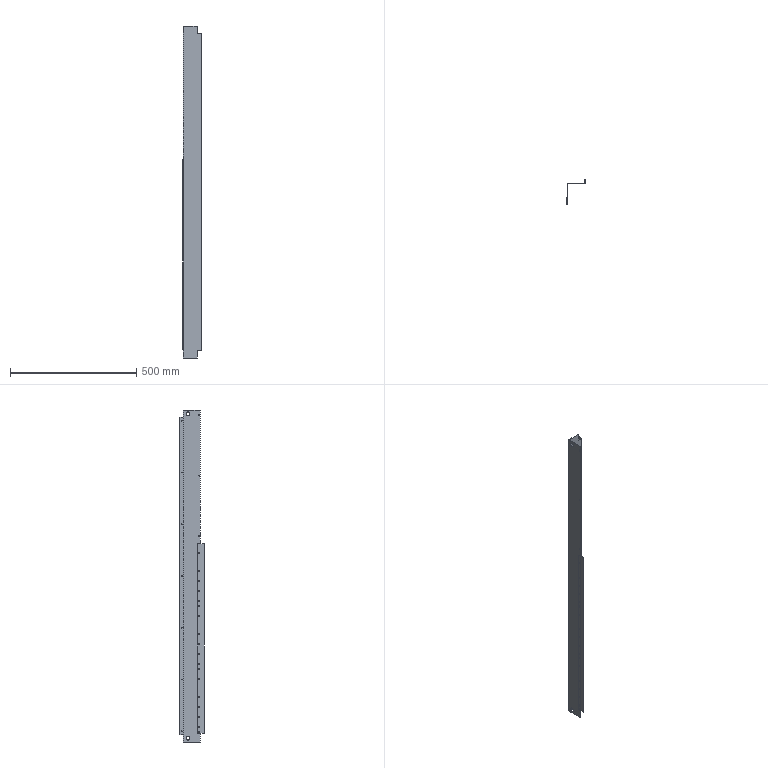Part | STEP file | 2 solids | 116 faces | box 73.2 x 96 x 1315 mm | volume 258859 mm3 | cylinder 96 | plane 20 | commonest cylinder face diameters 4.2 x72 3.2 x18 15 x4 6 x2